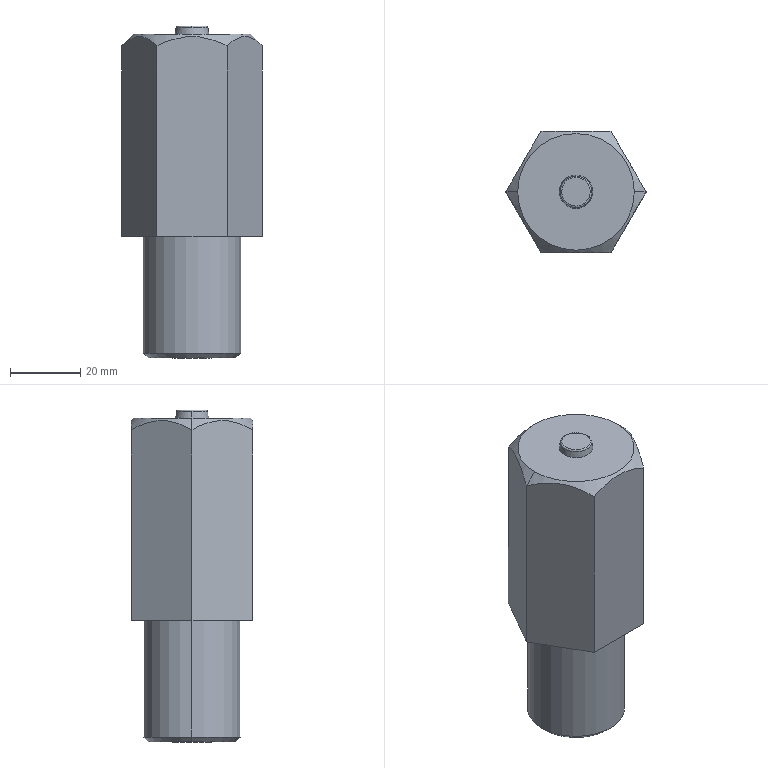Part | SolidWorks | features BaseBody 1 | 1 solid | 32 faces | box 39.97 x 34.615 x 94.615 mm | volume 79490 mm3 | plane 18 | cone 8 | cylinder 4 | spline 2 | commonest cylinder face diameters 11.347 x2 27.692 x2
STEP:
#1=CARTESIAN_POINT('',(-17.753,363.64,245.757));
#2=VERTEX_POINT('',#1);
#3=CARTESIAN_POINT('',(-13.229,359.115,245.757));
#4=VERTEX_POINT('',#3);
#5=CARTESIAN_POINT('',(-17.753,359.115,245.757));
#6=DIRECTION('',(0.,0.,-1.));
#7=DIRECTION('',(-1.,0.,0.));
#8=AXIS2_PLACEMENT_3D('',#5,#6,#7);
#9=CIRCLE('',#8,4.525);
#10=EDGE_CURVE('',#2,#4,#9,.T.);
#11=ORIENTED_EDGE('',*,*,#10,.F.);
#12=CARTESIAN_POINT('',(-17.753,363.183,246.154));
#13=VERTEX_POINT('',#12);
#14=CARTESIAN_POINT('',(-17.753,363.183,245.692));
#15=DIRECTION('',(1.,0.,0.));
#16=DIRECTION('',(0.,1.,0.));
#17=AXIS2_PLACEMENT_3D('',#14,#15,#16);
#18=CIRCLE('',#17,0.4615);
#19=EDGE_CURVE('',#2,#13,#18,.T.);
#20=ORIENTED_EDGE('',*,*,#19,.T.);
#21=CARTESIAN_POINT('',(-13.686,359.115,246.154));
#22=VERTEX_POINT('',#21);
#23=CARTESIAN_POINT('',(-17.753,363.183,246.154));
#24=CARTESIAN_POINT('',(-15.371,363.183,246.154));
#25=CARTESIAN_POINT('',(-13.686,361.498,246.154));
#26=CARTESIAN_POINT('',(-13.686,359.115,246.154));
#27=(BOUNDED_CURVE()B_SPLINE_CURVE(3,(#23,#24,#25,#26),.UNSPECIFIED.,.F.,.T.)B_SPLINE_CURVE_WITH_KNOTS((4,4),(0.,1.),.UNSPECIFIED.)CURVE()GEOMETRIC_REPRESENTATION_ITEM()RATIONAL_B_SPLINE_CURVE((1.,0.8047,0.8047,1.))REPRESENTATION_ITEM(''));
#28=EDGE_CURVE('',#13,#22,#27,.T.);
#29=ORIENTED_EDGE('',*,*,#28,.T.);
#30=CARTESIAN_POINT('',(-17.753,355.048,246.154));
#31=VERTEX_POINT('',#30);
#32=CARTESIAN_POINT('',(-13.686,359.115,246.154));
#33=CARTESIAN_POINT('',(-13.686,356.733,246.154));
#34=CARTESIAN_POINT('',(-15.371,355.048,246.154));
#35=CARTESIAN_POINT('',(-17.753,355.048,246.154));
#36=(BOUNDED_CURVE()B_SPLINE_CURVE(3,(#32,#33,#34,#35),.UNSPECIFIED.,.F.,.T.)B_SPLINE_CURVE_WITH_KNOTS((4,4),(0.,1.),.UNSPECIFIED.)CURVE()GEOMETRIC_REPRESENTATION_ITEM()RATIONAL_B_SPLINE_CURVE((1.,0.8047,0.8047,1.))REPRESENTATION_ITEM(''));
#37=EDGE_CURVE('',#22,#31,#36,.T.);
#38=ORIENTED_EDGE('',*,*,#37,.T.);
#39=CARTESIAN_POINT('',(-17.753,354.591,245.757));
#40=VERTEX_POINT('',#39);
#41=CARTESIAN_POINT('',(-17.753,355.048,245.692));
#42=DIRECTION('',(-1.,0.,0.));
#43=DIRECTION('',(0.,-1.,0.));
#44=AXIS2_PLACEMENT_3D('',#41,#42,#43);
#45=CIRCLE('',#44,0.4615);
#46=EDGE_CURVE('',#40,#31,#45,.T.);
#47=ORIENTED_EDGE('',*,*,#46,.F.);
#48=CARTESIAN_POINT('',(-17.753,359.115,245.757));
#49=DIRECTION('',(0.,0.,-1.));
#50=DIRECTION('',(-1.,0.,0.));
#51=AXIS2_PLACEMENT_3D('',#48,#49,#50);
#52=CIRCLE('',#51,4.525);
#53=EDGE_CURVE('',#4,#40,#52,.T.);
#54=ORIENTED_EDGE('',*,*,#53,.F.);
#55=EDGE_LOOP('',(#11,#20,#29,#38,#47,#54));
#56=FACE_OUTER_BOUND('',#55,.T.);
#57=CARTESIAN_POINT('',(-17.753,363.64,245.757));
#58=CARTESIAN_POINT('',(-8.704,363.64,245.757));
#59=CARTESIAN_POINT('',(-8.704,354.591,245.757));
#60=CARTESIAN_POINT('',(-17.753,354.591,245.757));
#61=CARTESIAN_POINT('',(-17.753,363.606,245.996));
#62=CARTESIAN_POINT('',(-8.771,363.606,245.996));
#63=CARTESIAN_POINT('',(-8.771,354.624,245.996));
#64=CARTESIAN_POINT('',(-17.753,354.624,245.996));
#65=CARTESIAN_POINT('',(-17.753,363.424,246.154));
#66=CARTESIAN_POINT('',(-9.136,363.424,246.154));
#67=CARTESIAN_POINT('',(-9.136,354.807,246.154));
#68=CARTESIAN_POINT('',(-17.753,354.807,246.154));
#69=CARTESIAN_POINT('',(-17.753,363.183,246.154));
#70=CARTESIAN_POINT('',(-9.618,363.183,246.154));
#71=CARTESIAN_POINT('',(-9.618,355.048,246.154));
#72=CARTESIAN_POINT('',(-17.753,355.048,246.154));
#73=(BOUNDED_SURFACE()B_SPLINE_SURFACE(3,3,((#57,#58,#59,#60),(#61,#62,#63,#64),(#65,#66,#67,#68),(#69,#70,#71,#72)),.UNSPECIFIED.,.F.,.F.,.T.)B_SPLINE_SURFACE_WITH_KNOTS((4,4),(4,4),(0.,1.),(0.,1.),.UNSPECIFIED.)GEOMETRIC_REPRESENTATION_ITEM()RATIONAL_B_SPLINE_SURFACE(((1.,0.3333,0.3333,1.),(0.8365,0.2788,0.2788,0.8365),(0.8365,0.2788,0.2788,0.8365),(1.,0.3333,0.3333,1.)))REPRESENTATION_ITEM('')SURFACE());
#74=ADVANCED_FACE('',(#56),#73,.T.);
#75=CARTESIAN_POINT('',(-3.907,359.115,152.954));
#76=VERTEX_POINT('',#75);
#77=CARTESIAN_POINT('',(-31.6,359.115,152.954));
#78=VERTEX_POINT('',#77);
#79=CARTESIAN_POINT('',(-17.753,359.115,152.954));
#80=DIRECTION('',(0.,0.,1.));
#81=DIRECTION('',(1.,0.,0.));
#82=AXIS2_PLACEMENT_3D('',#79,#80,#81);
#83=CIRCLE('',#82,13.846);
#84=EDGE_CURVE('',#76,#78,#83,.T.);
#85=ORIENTED_EDGE('',*,*,#84,.T.);
#86=CARTESIAN_POINT('',(-31.6,359.115,186.154));
#87=VERTEX_POINT('',#86);
#88=CARTESIAN_POINT('',(-31.6,359.115,151.538));
#89=DIRECTION('',(0.,0.,1.));
#90=VECTOR('',#89,1000.);
#91=LINE('',#88,#90);
#92=EDGE_CURVE('',#78,#87,#91,.T.);
#93=ORIENTED_EDGE('',*,*,#92,.T.);
#94=CARTESIAN_POINT('',(-3.907,359.115,186.154));
#95=VERTEX_POINT('',#94);
#96=CARTESIAN_POINT('',(-17.753,359.115,186.154));
#97=DIRECTION('',(0.,0.,-1.));
#98=DIRECTION('',(1.,0.,0.));
#99=AXIS2_PLACEMENT_3D('',#96,#97,#98);
#100=CIRCLE('',#99,13.846);
#101=EDGE_CURVE('',#87,#95,#100,.T.);
#102=ORIENTED_EDGE('',*,*,#101,.T.);
#103=CARTESIAN_POINT('',(-3.907,359.115,151.538));
#104=DIRECTION('',(0.,0.,1.));
#105=VECTOR('',#104,1000.);
#106=LINE('',#103,#105);
#107=EDGE_CURVE('',#76,#95,#106,.T.);
#108=ORIENTED_EDGE('',*,*,#107,.F.);
#109=EDGE_LOOP('',(#85,#93,#102,#108));
#110=FACE_OUTER_BOUND('',#109,.T.);
#111=CARTESIAN_POINT('',(-17.753,359.115,151.538));
#112=DIRECTION('',(0.,0.,1.));
#113=DIRECTION('',(1.,0.,0.));
#114=AXIS2_PLACEMENT_3D('',#111,#112,#113);
#115=CYLINDRICAL_SURFACE('',#114,13.846);
#116=ADVANCED_FACE('',(#110),#115,.T.);
#117=CARTESIAN_POINT('',(-5.323,359.115,151.538));
#118=VERTEX_POINT('',#117);
#119=CARTESIAN_POINT('',(-30.184,359.115,151.538));
#120=VERTEX_POINT('',#119);
#121=CARTESIAN_POINT('',(-17.753,359.115,151.538));
#122=DIRECTION('',(0.,0.,1.));
#123=DIRECTION('',(1.,0.,0.));
#124=AXIS2_PLACEMENT_3D('',#121,#122,#123);
#125=CIRCLE('',#124,12.43);
#126=EDGE_CURVE('',#118,#120,#125,.T.);
#127=ORIENTED_EDGE('',*,*,#126,.T.);
#128=CARTESIAN_POINT('',(-31.6,359.115,152.954));
#129=DIRECTION('',(-0.7071,0.,0.7071));
#130=VECTOR('',#129,1000.);
#131=LINE('',#128,#130);
#132=EDGE_CURVE('',#120,#78,#131,.T.);
#133=ORIENTED_EDGE('',*,*,#132,.T.);
#134=ORIENTED_EDGE('',*,*,#84,.F.);
#135=CARTESIAN_POINT('',(-3.907,359.115,152.954));
#136=DIRECTION('',(0.7071,0.,0.7071));
#137=VECTOR('',#136,1000.);
#138=LINE('',#135,#137);
#139=EDGE_CURVE('',#118,#76,#138,.T.);
#140=ORIENTED_EDGE('',*,*,#139,.F.);
#141=EDGE_LOOP('',(#127,#133,#134,#140));
#142=FACE_OUTER_BOUND('',#141,.T.);
#143=CARTESIAN_POINT('',(-17.753,359.115,152.954));
#144=DIRECTION('',(0.,0.,1.));
#145=DIRECTION('',(1.,0.,0.));
#146=AXIS2_PLACEMENT_3D('',#143,#144,#145);
#147=CONICAL_SURFACE('',#146,13.846,0.7854);
#148=ADVANCED_FACE('',(#142),#147,.T.);
#149=CARTESIAN_POINT('',(-34.369,359.115,243.846));
#150=VERTEX_POINT('',#149);
#151=CARTESIAN_POINT('',(-1.138,359.115,243.846));
#152=VERTEX_POINT('',#151);
#153=CARTESIAN_POINT('',(-17.753,359.115,243.846));
#154=DIRECTION('',(0.,0.,-1.));
#155=DIRECTION('',(-1.,0.,0.));
#156=AXIS2_PLACEMENT_3D('',#153,#154,#155);
#157=CIRCLE('',#156,16.615);
#158=EDGE_CURVE('',#150,#152,#157,.T.);
#159=ORIENTED_EDGE('',*,*,#158,.T.);
#160=CARTESIAN_POINT('',(2.232,359.115,240.476));
#161=VERTEX_POINT('',#160);
#162=CARTESIAN_POINT('',(2.252,359.115,240.456));
#163=DIRECTION('',(0.7071,0.,-0.7071));
#164=VECTOR('',#163,1000.);
#165=LINE('',#162,#164);
#166=EDGE_CURVE('',#152,#161,#165,.T.);
#167=ORIENTED_EDGE('',*,*,#166,.T.);
#168=CARTESIAN_POINT('',(-7.761,376.423,240.476));
#169=VERTEX_POINT('',#168);
#170=CARTESIAN_POINT('',(-7.761,376.423,240.476));
#171=CARTESIAN_POINT('',(-6.98,375.071,241.257));
#172=CARTESIAN_POINT('',(-6.182,373.688,241.921));
#173=CARTESIAN_POINT('',(-4.941,371.54,242.632));
#174=CARTESIAN_POINT('',(-4.521,370.811,242.821));
#175=CARTESIAN_POINT('',(-3.876,369.695,243.017));
#176=CARTESIAN_POINT('',(-3.659,369.319,243.067));
#177=CARTESIAN_POINT('',(-3.22,368.559,243.135));
#178=CARTESIAN_POINT('',(-3.001,368.179,243.153));
#179=CARTESIAN_POINT('',(-1.911,366.29,243.158));
#180=CARTESIAN_POINT('',(-1.053,364.805,242.893));
#181=CARTESIAN_POINT('',(0.6378,361.876,241.935));
#182=CARTESIAN_POINT('',(1.446,360.476,241.262));
#183=CARTESIAN_POINT('',(2.232,359.115,240.476));
#184=B_SPLINE_CURVE_WITH_KNOTS('',3,(#170,#171,#172,#173,#174,#175,#176,#177,#178,#179,#180,#181,#182,#183),.UNSPECIFIED.,.F.,.F.,(4,2,2,2,2,2,4),(0.,0.005161,0.007741,0.009032,0.01032,0.01548,0.02064),.UNSPECIFIED.);
#185=EDGE_CURVE('',#169,#161,#184,.T.);
#186=ORIENTED_EDGE('',*,*,#185,.F.);
#187=CARTESIAN_POINT('',(-27.746,376.423,240.476));
#188=VERTEX_POINT('',#187);
#189=CARTESIAN_POINT('',(-27.746,376.423,240.476));
#190=CARTESIAN_POINT('',(-26.185,376.423,241.257));
#191=CARTESIAN_POINT('',(-24.588,376.423,241.921));
#192=CARTESIAN_POINT('',(-22.107,376.423,242.632));
#193=CARTESIAN_POINT('',(-21.266,376.423,242.821));
#194=CARTESIAN_POINT('',(-19.977,376.423,243.017));
#195=CARTESIAN_POINT('',(-19.543,376.423,243.067));
#196=CARTESIAN_POINT('',(-18.665,376.423,243.135));
#197=CARTESIAN_POINT('',(-18.226,376.423,243.153));
#198=CARTESIAN_POINT('',(-16.046,376.423,243.158));
#199=CARTESIAN_POINT('',(-14.331,376.423,242.893));
#200=CARTESIAN_POINT('',(-10.949,376.423,241.935));
#201=CARTESIAN_POINT('',(-9.332,376.423,241.262));
#202=CARTESIAN_POINT('',(-7.761,376.423,240.476));
#203=B_SPLINE_CURVE_WITH_KNOTS('',3,(#189,#190,#191,#192,#193,#194,#195,#196,#197,#198,#199,#200,#201,#202),.UNSPECIFIED.,.F.,.F.,(4,2,2,2,2,2,4),(0.,0.005161,0.007741,0.009032,0.01032,0.01548,0.02064),.UNSPECIFIED.);
#204=EDGE_CURVE('',#188,#169,#203,.T.);
#205=ORIENTED_EDGE('',*,*,#204,.F.);
#206=CARTESIAN_POINT('',(-37.739,359.115,240.476));
#207=VERTEX_POINT('',#206);
#208=CARTESIAN_POINT('',(-37.739,359.115,240.476));
#209=CARTESIAN_POINT('',(-36.958,360.468,241.257));
#210=CARTESIAN_POINT('',(-36.16,361.851,241.921));
#211=CARTESIAN_POINT('',(-34.919,363.999,242.632));
#212=CARTESIAN_POINT('',(-34.499,364.728,242.821));
#213=CARTESIAN_POINT('',(-33.854,365.844,243.017));
#214=CARTESIAN_POINT('',(-33.637,366.219,243.067));
#215=CARTESIAN_POINT('',(-33.198,366.98,243.135));
#216=CARTESIAN_POINT('',(-32.979,367.36,243.153));
#217=CARTESIAN_POINT('',(-31.888,369.248,243.158));
#218=CARTESIAN_POINT('',(-31.031,370.733,242.893));
#219=CARTESIAN_POINT('',(-29.34,373.662,241.935));
#220=CARTESIAN_POINT('',(-28.531,375.063,241.262));
#221=CARTESIAN_POINT('',(-27.746,376.423,240.476));
#222=B_SPLINE_CURVE_WITH_KNOTS('',3,(#208,#209,#210,#211,#212,#213,#214,#215,#216,#217,#218,#219,#220,#221),.UNSPECIFIED.,.F.,.F.,(4,2,2,2,2,2,4),(0.,0.005161,0.007741,0.009032,0.01032,0.01548,0.02064),.UNSPECIFIED.);
#223=EDGE_CURVE('',#207,#188,#222,.T.);
#224=ORIENTED_EDGE('',*,*,#223,.F.);
#225=CARTESIAN_POINT('',(-37.759,359.115,240.456));
#226=DIRECTION('',(-0.7071,0.,-0.7071));
#227=VECTOR('',#226,1000.);
#228=LINE('',#225,#227);
#229=EDGE_CURVE('',#150,#207,#228,.T.);
#230=ORIENTED_EDGE('',*,*,#229,.F.);
#231=EDGE_LOOP('',(#159,#167,#186,#205,#224,#230));
#232=FACE_OUTER_BOUND('',#231,.T.);
#233=CARTESIAN_POINT('',(-17.753,359.115,240.456));
#234=DIRECTION('',(0.,0.,-1.));
#235=DIRECTION('',(-1.,0.,0.));
#236=AXIS2_PLACEMENT_3D('',#233,#234,#235);
#237=CONICAL_SURFACE('',#236,20.005,0.7854);
#238=ADVANCED_FACE('',(#232),#237,.T.);
#239=CARTESIAN_POINT('',(-12.08,359.115,151.538));
#240=VERTEX_POINT('',#239);
#241=CARTESIAN_POINT('',(-23.427,359.115,151.538));
#242=VERTEX_POINT('',#241);
#243=CARTESIAN_POINT('',(-17.753,359.115,151.538));
#244=DIRECTION('',(0.,0.,-1.));
#245=DIRECTION('',(1.,0.,0.));
#246=AXIS2_PLACEMENT_3D('',#243,#244,#245);
#247=CIRCLE('',#246,5.673);
#248=EDGE_CURVE('',#240,#242,#247,.T.);
#249=ORIENTED_EDGE('',*,*,#248,.T.);
#250=CARTESIAN_POINT('',(-23.427,359.115,160.935));
#251=VERTEX_POINT('',#250);
#252=CARTESIAN_POINT('',(-23.427,359.115,151.538));
#253=DIRECTION('',(0.,0.,1.));
#254=VECTOR('',#253,1000.);
#255=LINE('',#252,#254);
#256=EDGE_CURVE('',#242,#251,#255,.T.);
#257=ORIENTED_EDGE('',*,*,#256,.T.);
#258=CARTESIAN_POINT('',(-12.08,359.115,160.935));
#259=VERTEX_POINT('',#258);
#260=CARTESIAN_POINT('',(-17.753,359.115,160.935));
#261=DIRECTION('',(0.,0.,-1.));
#262=DIRECTION('',(1.,0.,0.));
#263=AXIS2_PLACEMENT_3D('',#260,#261,#262);
#264=CIRCLE('',#263,5.673);
#265=EDGE_CURVE('',#259,#251,#264,.T.);
#266=ORIENTED_EDGE('',*,*,#265,.F.);
#267=CARTESIAN_POINT('',(-12.08,359.115,151.538));
#268=DIRECTION('',(0.,0.,1.));
#269=VECTOR('',#268,1000.);
#270=LINE('',#267,#269);
#271=EDGE_CURVE('',#240,#259,#270,.T.);
#272=ORIENTED_EDGE('',*,*,#271,.F.);
#273=EDGE_LOOP('',(#249,#257,#266,#272));
#274=FACE_OUTER_BOUND('',#273,.T.);
#275=CARTESIAN_POINT('',(-17.753,359.115,151.538));
#276=DIRECTION('',(0.,0.,1.));
#277=DIRECTION('',(1.,0.,0.));
#278=AXIS2_PLACEMENT_3D('',#275,#276,#277);
#279=CYLINDRICAL_SURFACE('',#278,5.673);
#280=ADVANCED_FACE('',(#274),#279,.F.);
#281=CARTESIAN_POINT('',(-12.246,359.115,160.769));
#282=VERTEX_POINT('',#281);
#283=CARTESIAN_POINT('',(-23.261,359.115,160.769));
#284=VERTEX_POINT('',#283);
#285=CARTESIAN_POINT('',(-17.753,359.115,160.769));
#286=DIRECTION('',(0.,0.,1.));
#287=DIRECTION('',(1.,0.,0.));
#288=AXIS2_PLACEMENT_3D('',#285,#286,#287);
#289=CIRCLE('',#288,5.507);
#290=EDGE_CURVE('',#282,#284,#289,.T.);
#291=ORIENTED_EDGE('',*,*,#290,.T.);
#292=CARTESIAN_POINT('',(-23.427,359.115,160.935));
#293=DIRECTION('',(-0.7071,0.,0.7071));
#294=VECTOR('',#293,1000.);
#295=LINE('',#292,#294);
#296=EDGE_CURVE('',#284,#251,#295,.T.);
#297=ORIENTED_EDGE('',*,*,#296,.T.);
#298=CARTESIAN_POINT('',(-17.753,359.115,160.935));
#299=DIRECTION('',(0.,0.,-1.));
#300=DIRECTION('',(1.,0.,0.));
#301=AXIS2_PLACEMENT_3D('',#298,#299,#300);
#302=CIRCLE('',#301,5.673);
#303=EDGE_CURVE('',#251,#259,#302,.T.);
#304=ORIENTED_EDGE('',*,*,#303,.T.);
#305=CARTESIAN_POINT('',(-12.08,359.115,160.935));
#306=DIRECTION('',(0.7071,0.,0.7071));
#307=VECTOR('',#306,1000.);
#308=LINE('',#305,#307);
#309=EDGE_CURVE('',#282,#259,#308,.T.);
#310=ORIENTED_EDGE('',*,*,#309,.F.);
#311=EDGE_LOOP('',(#291,#297,#304,#310));
#312=FACE_OUTER_BOUND('',#311,.T.);
#313=CARTESIAN_POINT('',(-17.753,359.115,160.935));
#314=DIRECTION('',(0.,0.,1.));
#315=DIRECTION('',(1.,0.,0.));
#316=AXIS2_PLACEMENT_3D('',#313,#314,#315);
#317=CONICAL_SURFACE('',#316,5.673,0.7854);
#318=ADVANCED_FACE('',(#312),#317,.T.);
#319=CARTESIAN_POINT('',(-22.278,359.115,245.757));
#320=VERTEX_POINT('',#319);
#321=CARTESIAN_POINT('',(-17.753,359.115,245.757));
#322=DIRECTION('',(0.,0.,-1.));
#323=DIRECTION('',(-1.,0.,0.));
#324=AXIS2_PLACEMENT_3D('',#321,#322,#323);
#325=CIRCLE('',#324,4.525);
#326=EDGE_CURVE('',#320,#2,#325,.T.);
#327=ORIENTED_EDGE('',*,*,#326,.T.);
#328=ORIENTED_EDGE('',*,*,#10,.T.);
#329=CARTESIAN_POINT('',(-12.96,359.115,243.846));
#330=VERTEX_POINT('',#329);
#331=CARTESIAN_POINT('',(-12.96,359.115,243.846));
#332=DIRECTION('',(0.1392,0.,-0.9903));
#333=VECTOR('',#332,1000.);
#334=LINE('',#331,#333);
#335=EDGE_CURVE('',#4,#330,#334,.T.);
#336=ORIENTED_EDGE('',*,*,#335,.T.);
#337=CARTESIAN_POINT('',(-22.547,359.115,243.846));
#338=VERTEX_POINT('',#337);
#339=CARTESIAN_POINT('',(-17.753,359.115,243.846));
#340=DIRECTION('',(0.,0.,1.));
#341=DIRECTION('',(-1.,0.,0.));
#342=AXIS2_PLACEMENT_3D('',#339,#340,#341);
#343=CIRCLE('',#342,4.793);
#344=EDGE_CURVE('',#330,#338,#343,.T.);
#345=ORIENTED_EDGE('',*,*,#344,.T.);
#346=CARTESIAN_POINT('',(-22.547,359.115,243.846));
#347=DIRECTION('',(-0.1392,0.,-0.9903));
#348=VECTOR('',#347,1000.);
#349=LINE('',#346,#348);
#350=EDGE_CURVE('',#320,#338,#349,.T.);
#351=ORIENTED_EDGE('',*,*,#350,.F.);
#352=EDGE_LOOP('',(#327,#328,#336,#345,#351));
#353=FACE_OUTER_BOUND('',#352,.T.);
#354=CARTESIAN_POINT('',(-17.753,359.115,243.846));
#355=DIRECTION('',(0.,0.,-1.));
#356=DIRECTION('',(-1.,0.,0.));
#357=AXIS2_PLACEMENT_3D('',#354,#355,#356);
#358=CONICAL_SURFACE('',#357,4.793,0.1396);
#359=ADVANCED_FACE('',(#353),#358,.T.);
#360=ORIENTED_EDGE('',*,*,#92,.F.);
#361=CARTESIAN_POINT('',(-17.753,359.115,152.954));
#362=DIRECTION('',(0.,0.,1.));
#363=DIRECTION('',(1.,0.,0.));
#364=AXIS2_PLACEMENT_3D('',#361,#362,#363);
#365=CIRCLE('',#364,13.846);
#366=EDGE_CURVE('',#78,#76,#365,.T.);
#367=ORIENTED_EDGE('',*,*,#366,.T.);
#368=ORIENTED_EDGE('',*,*,#107,.T.);
#369=CARTESIAN_POINT('',(-17.753,359.115,186.154));
#370=DIRECTION('',(0.,0.,-1.));
#371=DIRECTION('',(1.,0.,0.));
#372=AXIS2_PLACEMENT_3D('',#369,#370,#371);
#373=CIRCLE('',#372,13.846);
#374=EDGE_CURVE('',#95,#87,#373,.T.);
#375=ORIENTED_EDGE('',*,*,#374,.T.);
#376=EDGE_LOOP('',(#360,#367,#368,#375));
#377=FACE_OUTER_BOUND('',#376,.T.);
#378=CARTESIAN_POINT('',(-17.753,359.115,151.538));
#379=DIRECTION('',(0.,0.,1.));
#380=DIRECTION('',(1.,0.,0.));
#381=AXIS2_PLACEMENT_3D('',#378,#379,#380);
#382=CYLINDRICAL_SURFACE('',#381,13.846);
#383=ADVANCED_FACE('',(#377),#382,.T.);
#384=ORIENTED_EDGE('',*,*,#374,.F.);
#385=ORIENTED_EDGE('',*,*,#101,.F.);
#386=EDGE_LOOP('',(#384,#385));
#387=FACE_BOUND('',#386,.T.);
#388=CARTESIAN_POINT('',(-7.761,376.423,186.154));
#389=VERTEX_POINT('',#388);
#390=CARTESIAN_POINT('',(-27.746,376.423,186.154));
#391=VERTEX_POINT('',#390);
#392=CARTESIAN_POINT('',(-17.753,376.423,186.154));
#393=DIRECTION('',(-1.,0.,0.));
#394=VECTOR('',#393,1000.);
#395=LINE('',#392,#394);
#396=EDGE_CURVE('',#389,#391,#395,.T.);
#397=ORIENTED_EDGE('',*,*,#396,.F.);
#398=CARTESIAN_POINT('',(2.232,359.115,186.154));
#399=VERTEX_POINT('',#398);
#400=CARTESIAN_POINT('',(2.232,359.115,186.154));
#401=DIRECTION('',(-0.5,0.866,0.));
#402=VECTOR('',#401,1000.);
#403=LINE('',#400,#402);
#404=EDGE_CURVE('',#399,#389,#403,.T.);
#405=ORIENTED_EDGE('',*,*,#404,.F.);
#406=CARTESIAN_POINT('',(-7.761,341.808,186.154));
#407=VERTEX_POINT('',#406);
#408=CARTESIAN_POINT('',(-7.761,341.808,186.154));
#409=DIRECTION('',(0.5,0.866,0.));
#410=VECTOR('',#409,1000.);
#411=LINE('',#408,#410);
#412=EDGE_CURVE('',#407,#399,#411,.T.);
#413=ORIENTED_EDGE('',*,*,#412,.F.);
#414=CARTESIAN_POINT('',(-27.746,341.808,186.154));
#415=VERTEX_POINT('',#414);
#416=CARTESIAN_POINT('',(-17.753,341.808,186.154));
#417=DIRECTION('',(1.,0.,0.));
#418=VECTOR('',#417,1000.);
#419=LINE('',#416,#418);
#420=EDGE_CURVE('',#415,#407,#419,.T.);
#421=ORIENTED_EDGE('',*,*,#420,.F.);
#422=CARTESIAN_POINT('',(-37.739,359.115,186.154));
#423=VERTEX_POINT('',#422);
#424=CARTESIAN_POINT('',(-37.739,359.115,186.154));
#425=DIRECTION('',(0.5,-0.866,0.));
#426=VECTOR('',#425,1000.);
#427=LINE('',#424,#426);
#428=EDGE_CURVE('',#423,#415,#427,.T.);
#429=ORIENTED_EDGE('',*,*,#428,.F.);
#430=CARTESIAN_POINT('',(-27.746,376.423,186.154));
#431=DIRECTION('',(-0.5,-0.866,0.));
#432=VECTOR('',#431,1000.);
#433=LINE('',#430,#432);
#434=EDGE_CURVE('',#391,#423,#433,.T.);
#435=ORIENTED_EDGE('',*,*,#434,.F.);
#436=EDGE_LOOP('',(#397,#405,#413,#421,#429,#435));
#437=FACE_OUTER_BOUND('',#436,.T.);
#438=CARTESIAN_POINT('',(-17.753,339.039,186.154));
#439=DIRECTION('',(0.,0.,1.));
#440=DIRECTION('',(1.,0.,0.));
#441=AXIS2_PLACEMENT_3D('',#438,#439,#440);
#442=PLANE('',#441);
#443=ADVANCED_FACE('',(#387,#437),#442,.F.);
#444=ORIENTED_EDGE('',*,*,#132,.F.);
#445=CARTESIAN_POINT('',(-17.753,359.115,151.538));
#446=DIRECTION('',(0.,0.,1.));
#447=DIRECTION('',(1.,0.,0.));
#448=AXIS2_PLACEMENT_3D('',#445,#446,#447);
#449=CIRCLE('',#448,12.43);
#450=EDGE_CURVE('',#120,#118,#449,.T.);
#451=ORIENTED_EDGE('',*,*,#450,.T.);
#452=ORIENTED_EDGE('',*,*,#139,.T.);
#453=ORIENTED_EDGE('',*,*,#366,.F.);
#454=EDGE_LOOP('',(#444,#451,#452,#453));
#455=FACE_OUTER_BOUND('',#454,.T.);
#456=CARTESIAN_POINT('',(-17.753,359.115,152.954));
#457=DIRECTION('',(0.,0.,1.));
#458=DIRECTION('',(1.,0.,0.));
#459=AXIS2_PLACEMENT_3D('',#456,#457,#458);
#460=CONICAL_SURFACE('',#459,13.846,0.7854);
#461=ADVANCED_FACE('',(#455),#460,.T.);
#462=CARTESIAN_POINT('',(-27.746,376.423,186.154));
#463=DIRECTION('',(0.,0.,-1.));
#464=VECTOR('',#463,1000.);
#465=LINE('',#462,#464);
#466=EDGE_CURVE('',#188,#391,#465,.T.);
#467=ORIENTED_EDGE('',*,*,#466,.T.);
#468=ORIENTED_EDGE('',*,*,#434,.T.);
#469=CARTESIAN_POINT('',(-37.739,359.115,186.154));
#470=DIRECTION('',(0.,0.,1.));
#471=VECTOR('',#470,1000.);
#472=LINE('',#469,#471);
#473=EDGE_CURVE('',#423,#207,#472,.T.);
#474=ORIENTED_EDGE('',*,*,#473,.T.);
#475=ORIENTED_EDGE('',*,*,#223,.T.);
#476=EDGE_LOOP('',(#467,#468,#474,#475));
#477=FACE_OUTER_BOUND('',#476,.T.);
#478=CARTESIAN_POINT('',(-27.746,376.423,186.154));
#479=DIRECTION('',(-0.866,0.5,0.));
#480=DIRECTION('',(-0.5,-0.866,0.));
#481=AXIS2_PLACEMENT_3D('',#478,#479,#480);
#482=PLANE('',#481);
#483=ADVANCED_FACE('',(#477),#482,.T.);
#484=CARTESIAN_POINT('',(-7.761,376.423,186.154));
#485=DIRECTION('',(0.,0.,-1.));
#486=VECTOR('',#485,1000.);
#487=LINE('',#484,#486);
#488=EDGE_CURVE('',#169,#389,#487,.T.);
#489=ORIENTED_EDGE('',*,*,#488,.T.);
#490=ORIENTED_EDGE('',*,*,#396,.T.);
#491=ORIENTED_EDGE('',*,*,#466,.F.);
#492=ORIENTED_EDGE('',*,*,#204,.T.);
#493=EDGE_LOOP('',(#489,#490,#491,#492));
#494=FACE_OUTER_BOUND('',#493,.T.);
#495=CARTESIAN_POINT('',(-7.761,376.423,186.154));
#496=DIRECTION('',(0.,1.,0.));
#497=DIRECTION('',(0.,0.,1.));
#498=AXIS2_PLACEMENT_3D('',#495,#496,#497);
#499=PLANE('',#498);
#500=ADVANCED_FACE('',(#494),#499,.T.);
#501=CARTESIAN_POINT('',(2.232,359.115,186.154));
#502=DIRECTION('',(0.,0.,-1.));
#503=VECTOR('',#502,1000.);
#504=LINE('',#501,#503);
#505=EDGE_CURVE('',#161,#399,#504,.T.);
#506=ORIENTED_EDGE('',*,*,#505,.T.);
#507=ORIENTED_EDGE('',*,*,#404,.T.);
#508=ORIENTED_EDGE('',*,*,#488,.F.);
#509=ORIENTED_EDGE('',*,*,#185,.T.);
#510=EDGE_LOOP('',(#506,#507,#508,#509));
#511=FACE_OUTER_BOUND('',#510,.T.);
#512=CARTESIAN_POINT('',(2.232,359.115,186.154));
#513=DIRECTION('',(0.866,0.5,0.));
#514=DIRECTION('',(-0.5,0.866,0.));
#515=AXIS2_PLACEMENT_3D('',#512,#513,#514);
#516=PLANE('',#515);
#517=ADVANCED_FACE('',(#511),#516,.T.);
#518=CARTESIAN_POINT('',(-7.761,341.808,240.476));
#519=VERTEX_POINT('',#518);
#520=CARTESIAN_POINT('',(-7.761,341.808,186.154));
#521=DIRECTION('',(0.,0.,-1.));
#522=VECTOR('',#521,1000.);
#523=LINE('',#520,#522);
#524=EDGE_CURVE('',#519,#407,#523,.T.);
#525=ORIENTED_EDGE('',*,*,#524,.T.);
#526=ORIENTED_EDGE('',*,*,#412,.T.);
#527=ORIENTED_EDGE('',*,*,#505,.F.);
#528=CARTESIAN_POINT('',(2.232,359.115,240.476));
#529=CARTESIAN_POINT('',(1.451,357.763,241.257));
#530=CARTESIAN_POINT('',(0.6526,356.38,241.921));
#531=CARTESIAN_POINT('',(-0.5878,354.232,242.632));
#532=CARTESIAN_POINT('',(-1.008,353.503,242.821));
#533=CARTESIAN_POINT('',(-1.653,352.387,243.017));
#534=CARTESIAN_POINT('',(-1.87,352.011,243.067));
#535=CARTESIAN_POINT('',(-2.309,351.251,243.135));
#536=CARTESIAN_POINT('',(-2.528,350.871,243.153));
#537=CARTESIAN_POINT('',(-3.619,348.983,243.158));
#538=CARTESIAN_POINT('',(-4.476,347.497,242.893));
#539=CARTESIAN_POINT('',(-6.167,344.569,241.935));
#540=CARTESIAN_POINT('',(-6.976,343.168,241.262));
#541=CARTESIAN_POINT('',(-7.761,341.808,240.476));
#542=B_SPLINE_CURVE_WITH_KNOTS('',3,(#528,#529,#530,#531,#532,#533,#534,#535,#536,#537,#538,#539,#540,#541),.UNSPECIFIED.,.F.,.F.,(4,2,2,2,2,2,4),(0.,0.005161,0.007741,0.009032,0.01032,0.01548,0.02064),.UNSPECIFIED.);
#543=EDGE_CURVE('',#161,#519,#542,.T.);
#544=ORIENTED_EDGE('',*,*,#543,.T.);
#545=EDGE_LOOP('',(#525,#526,#527,#544));
#546=FACE_OUTER_BOUND('',#545,.T.);
#547=CARTESIAN_POINT('',(-7.761,341.808,186.154));
#548=DIRECTION('',(0.866,-0.5,0.));
#549=DIRECTION('',(0.5,0.866,0.));
#550=AXIS2_PLACEMENT_3D('',#547,#548,#549);
#551=PLANE('',#550);
#552=ADVANCED_FACE('',(#546),#551,.T.);
#553=CARTESIAN_POINT('',(-27.746,341.808,240.476));
#554=VERTEX_POINT('',#553);
#555=CARTESIAN_POINT('',(-27.746,341.808,186.154));
#556=DIRECTION('',(0.,0.,-1.));
#557=VECTOR('',#556,1000.);
#558=LINE('',#555,#557);
#559=EDGE_CURVE('',#554,#415,#558,.T.);
#560=ORIENTED_EDGE('',*,*,#559,.T.);
#561=ORIENTED_EDGE('',*,*,#420,.T.);
#562=ORIENTED_EDGE('',*,*,#524,.F.);
#563=CARTESIAN_POINT('',(-7.761,341.808,240.476));
#564=CARTESIAN_POINT('',(-9.322,341.808,241.257));
#565=CARTESIAN_POINT('',(-10.919,341.808,241.921));
#566=CARTESIAN_POINT('',(-13.4,341.808,242.632));
#567=CARTESIAN_POINT('',(-14.241,341.808,242.821));
#568=CARTESIAN_POINT('',(-15.53,341.808,243.017));
#569=CARTESIAN_POINT('',(-15.964,341.808,243.067));
#570=CARTESIAN_POINT('',(-16.842,341.808,243.135));
#571=CARTESIAN_POINT('',(-17.281,341.808,243.153));
#572=CARTESIAN_POINT('',(-19.461,341.808,243.158));
#573=CARTESIAN_POINT('',(-21.176,341.808,242.893));
#574=CARTESIAN_POINT('',(-24.558,341.808,241.935));
#575=CARTESIAN_POINT('',(-26.175,341.808,241.262));
#576=CARTESIAN_POINT('',(-27.746,341.808,240.476));
#577=B_SPLINE_CURVE_WITH_KNOTS('',3,(#563,#564,#565,#566,#567,#568,#569,#570,#571,#572,#573,#574,#575,#576),.UNSPECIFIED.,.F.,.F.,(4,2,2,2,2,2,4),(0.,0.005161,0.007741,0.009032,0.01032,0.01548,0.02064),.UNSPECIFIED.);
#578=EDGE_CURVE('',#519,#554,#577,.T.);
#579=ORIENTED_EDGE('',*,*,#578,.T.);
#580=EDGE_LOOP('',(#560,#561,#562,#579));
#581=FACE_OUTER_BOUND('',#580,.T.);
#582=CARTESIAN_POINT('',(-27.746,341.808,186.154));
#583=DIRECTION('',(0.,-1.,0.));
#584=DIRECTION('',(0.,0.,-1.));
#585=AXIS2_PLACEMENT_3D('',#582,#583,#584);
#586=PLANE('',#585);
#587=ADVANCED_FACE('',(#581),#586,.T.);
#588=ORIENTED_EDGE('',*,*,#473,.F.);
#589=ORIENTED_EDGE('',*,*,#428,.T.);
#590=ORIENTED_EDGE('',*,*,#559,.F.);
#591=CARTESIAN_POINT('',(-27.746,341.808,240.476));
#592=CARTESIAN_POINT('',(-28.527,343.16,241.257));
#593=CARTESIAN_POINT('',(-29.325,344.543,241.921));
#594=CARTESIAN_POINT('',(-30.566,346.691,242.632));
#595=CARTESIAN_POINT('',(-30.986,347.42,242.821));
#596=CARTESIAN_POINT('',(-31.631,348.536,243.017));
#597=CARTESIAN_POINT('',(-31.848,348.912,243.067));
#598=CARTESIAN_POINT('',(-32.286,349.672,243.135));
#599=CARTESIAN_POINT('',(-32.506,350.052,243.153));
#600=CARTESIAN_POINT('',(-33.596,351.941,243.158));
#601=CARTESIAN_POINT('',(-34.454,353.426,242.893));
#602=CARTESIAN_POINT('',(-36.145,356.355,241.935));
#603=CARTESIAN_POINT('',(-36.953,357.755,241.262));
#604=CARTESIAN_POINT('',(-37.739,359.115,240.476));
#605=B_SPLINE_CURVE_WITH_KNOTS('',3,(#591,#592,#593,#594,#595,#596,#597,#598,#599,#600,#601,#602,#603,#604),.UNSPECIFIED.,.F.,.F.,(4,2,2,2,2,2,4),(0.,0.005161,0.007741,0.009032,0.01032,0.01548,0.02064),.UNSPECIFIED.);
#606=EDGE_CURVE('',#554,#207,#605,.T.);
#607=ORIENTED_EDGE('',*,*,#606,.T.);
#608=EDGE_LOOP('',(#588,#589,#590,#607));
#609=FACE_OUTER_BOUND('',#608,.T.);
#610=CARTESIAN_POINT('',(-37.739,359.115,186.154));
#611=DIRECTION('',(-0.866,-0.5,0.));
#612=DIRECTION('',(0.5,-0.866,0.));
#613=AXIS2_PLACEMENT_3D('',#610,#611,#612);
#614=PLANE('',#613);
#615=ADVANCED_FACE('',(#609),#614,.T.);
#616=ORIENTED_EDGE('',*,*,#248,.F.);
#617=CARTESIAN_POINT('',(-17.753,359.115,151.538));
#618=DIRECTION('',(0.,0.,-1.));
#619=DIRECTION('',(1.,0.,0.));
#620=AXIS2_PLACEMENT_3D('',#617,#618,#619);
#621=CIRCLE('',#620,5.673);
#622=EDGE_CURVE('',#242,#240,#621,.T.);
#623=ORIENTED_EDGE('',*,*,#622,.F.);
#624=EDGE_LOOP('',(#616,#623));
#625=FACE_BOUND('',#624,.T.);
#626=ORIENTED_EDGE('',*,*,#126,.F.);
#627=ORIENTED_EDGE('',*,*,#450,.F.);
#628=EDGE_LOOP('',(#626,#627));
#629=FACE_OUTER_BOUND('',#628,.T.);
#630=CARTESIAN_POINT('',(-17.753,346.685,151.538));
#631=DIRECTION('',(0.,0.,1.));
#632=DIRECTION('',(1.,0.,0.));
#633=AXIS2_PLACEMENT_3D('',#630,#631,#632);
#634=PLANE('',#633);
#635=ADVANCED_FACE('',(#625,#629),#634,.F.);
#636=ORIENTED_EDGE('',*,*,#166,.F.);
#637=CARTESIAN_POINT('',(-17.753,359.115,243.846));
#638=DIRECTION('',(0.,0.,-1.));
#639=DIRECTION('',(-1.,0.,0.));
#640=AXIS2_PLACEMENT_3D('',#637,#638,#639);
#641=CIRCLE('',#640,16.615);
#642=EDGE_CURVE('',#152,#150,#641,.T.);
#643=ORIENTED_EDGE('',*,*,#642,.T.);
#644=ORIENTED_EDGE('',*,*,#229,.T.);
#645=ORIENTED_EDGE('',*,*,#606,.F.);
#646=ORIENTED_EDGE('',*,*,#578,.F.);
#647=ORIENTED_EDGE('',*,*,#543,.F.);
#648=EDGE_LOOP('',(#636,#643,#644,#645,#646,#647));
#649=FACE_OUTER_BOUND('',#648,.T.);
#650=CARTESIAN_POINT('',(-17.753,359.115,240.456));
#651=DIRECTION('',(0.,0.,-1.));
#652=DIRECTION('',(-1.,0.,0.));
#653=AXIS2_PLACEMENT_3D('',#650,#651,#652);
#654=CONICAL_SURFACE('',#653,20.005,0.7854);
#655=ADVANCED_FACE('',(#649),#654,.T.);
#656=ORIENTED_EDGE('',*,*,#256,.F.);
#657=ORIENTED_EDGE('',*,*,#622,.T.);
#658=ORIENTED_EDGE('',*,*,#271,.T.);
#659=ORIENTED_EDGE('',*,*,#303,.F.);
#660=EDGE_LOOP('',(#656,#657,#658,#659));
#661=FACE_OUTER_BOUND('',#660,.T.);
#662=CARTESIAN_POINT('',(-17.753,359.115,151.538));
#663=DIRECTION('',(0.,0.,1.));
#664=DIRECTION('',(1.,0.,0.));
#665=AXIS2_PLACEMENT_3D('',#662,#663,#664);
#666=CYLINDRICAL_SURFACE('',#665,5.673);
#667=ADVANCED_FACE('',(#661),#666,.F.);
#668=CARTESIAN_POINT('',(-17.753,359.115,243.846));
#669=DIRECTION('',(0.,0.,1.));
#670=DIRECTION('',(-1.,0.,0.));
#671=AXIS2_PLACEMENT_3D('',#668,#669,#670);
#672=CIRCLE('',#671,4.793);
#673=EDGE_CURVE('',#338,#330,#672,.T.);
#674=ORIENTED_EDGE('',*,*,#673,.F.);
#675=ORIENTED_EDGE('',*,*,#344,.F.);
#676=EDGE_LOOP('',(#674,#675));
#677=FACE_BOUND('',#676,.T.);
#678=ORIENTED_EDGE('',*,*,#158,.F.);
#679=ORIENTED_EDGE('',*,*,#642,.F.);
#680=EDGE_LOOP('',(#678,#679));
#681=FACE_OUTER_BOUND('',#680,.T.);
#682=CARTESIAN_POINT('',(-17.753,359.115,243.846));
#683=DIRECTION('',(0.,0.,-1.));
#684=DIRECTION('',(-1.,0.,0.));
#685=AXIS2_PLACEMENT_3D('',#682,#683,#684);
#686=PLANE('',#685);
#687=ADVANCED_FACE('',(#677,#681),#686,.F.);
#688=ORIENTED_EDGE('',*,*,#296,.F.);
#689=CARTESIAN_POINT('',(-17.753,359.115,160.769));
#690=DIRECTION('',(0.,0.,1.));
#691=DIRECTION('',(1.,0.,0.));
#692=AXIS2_PLACEMENT_3D('',#689,#690,#691);
#693=CIRCLE('',#692,5.507);
#694=EDGE_CURVE('',#284,#282,#693,.T.);
#695=ORIENTED_EDGE('',*,*,#694,.T.);
#696=ORIENTED_EDGE('',*,*,#309,.T.);
#697=ORIENTED_EDGE('',*,*,#265,.T.);
#698=EDGE_LOOP('',(#688,#695,#696,#697));
#699=FACE_OUTER_BOUND('',#698,.T.);
#700=CARTESIAN_POINT('',(-17.753,359.115,160.935));
#701=DIRECTION('',(0.,0.,1.));
#702=DIRECTION('',(1.,0.,0.));
#703=AXIS2_PLACEMENT_3D('',#700,#701,#702);
#704=CONICAL_SURFACE('',#703,5.673,0.7854);
#705=ADVANCED_FACE('',(#699),#704,.T.);
#706=ORIENTED_EDGE('',*,*,#335,.F.);
#707=ORIENTED_EDGE('',*,*,#53,.T.);
#708=CARTESIAN_POINT('',(-17.753,359.115,245.757));
#709=DIRECTION('',(0.,0.,-1.));
#710=DIRECTION('',(-1.,0.,0.));
#711=AXIS2_PLACEMENT_3D('',#708,#709,#710);
#712=CIRCLE('',#711,4.525);
#713=EDGE_CURVE('',#40,#320,#712,.T.);
#714=ORIENTED_EDGE('',*,*,#713,.T.);
#715=ORIENTED_EDGE('',*,*,#350,.T.);
#716=ORIENTED_EDGE('',*,*,#673,.T.);
#717=EDGE_LOOP('',(#706,#707,#714,#715,#716));
#718=FACE_OUTER_BOUND('',#717,.T.);
#719=CARTESIAN_POINT('',(-17.753,359.115,243.846));
#720=DIRECTION('',(0.,0.,-1.));
#721=DIRECTION('',(-1.,0.,0.));
#722=AXIS2_PLACEMENT_3D('',#719,#720,#721);
#723=CONICAL_SURFACE('',#722,4.793,0.1396);
#724=ADVANCED_FACE('',(#718),#723,.T.);
#725=CARTESIAN_POINT('',(-17.753,363.112,160.769));
#726=VERTEX_POINT('',#725);
#727=CARTESIAN_POINT('',(-14.292,361.114,160.769));
#728=VERTEX_POINT('',#727);
#729=CARTESIAN_POINT('',(-17.753,363.112,160.769));
#730=DIRECTION('',(0.866,-0.5,0.));
#731=VECTOR('',#730,1000.);
#732=LINE('',#729,#731);
#733=EDGE_CURVE('',#726,#728,#732,.T.);
#734=ORIENTED_EDGE('',*,*,#733,.F.);
#735=CARTESIAN_POINT('',(-21.215,361.114,160.769));
#736=VERTEX_POINT('',#735);
#737=CARTESIAN_POINT('',(-21.215,361.114,160.769));
#738=DIRECTION('',(0.866,0.5,0.));
#739=VECTOR('',#738,1000.);
#740=LINE('',#737,#739);
#741=EDGE_CURVE('',#736,#726,#740,.T.);
#742=ORIENTED_EDGE('',*,*,#741,.F.);
#743=CARTESIAN_POINT('',(-21.215,357.117,160.769));
#744=VERTEX_POINT('',#743);
#745=CARTESIAN_POINT('',(-21.215,353.608,160.769));
#746=DIRECTION('',(0.,1.,0.));
#747=VECTOR('',#746,1000.);
#748=LINE('',#745,#747);
#749=EDGE_CURVE('',#744,#736,#748,.T.);
#750=ORIENTED_EDGE('',*,*,#749,.F.);
#751=CARTESIAN_POINT('',(-17.753,355.118,160.769));
#752=VERTEX_POINT('',#751);
#753=CARTESIAN_POINT('',(-17.753,355.118,160.769));
#754=DIRECTION('',(-0.866,0.5,0.));
#755=VECTOR('',#754,1000.);
#756=LINE('',#753,#755);
#757=EDGE_CURVE('',#752,#744,#756,.T.);
#758=ORIENTED_EDGE('',*,*,#757,.F.);
#759=CARTESIAN_POINT('',(-14.292,357.117,160.769));
#760=VERTEX_POINT('',#759);
#761=CARTESIAN_POINT('',(-14.292,357.117,160.769));
#762=DIRECTION('',(-0.866,-0.5,0.));
#763=VECTOR('',#762,1000.);
#764=LINE('',#761,#763);
#765=EDGE_CURVE('',#760,#752,#764,.T.);
#766=ORIENTED_EDGE('',*,*,#765,.F.);
#767=CARTESIAN_POINT('',(-14.292,353.608,160.769));
#768=DIRECTION('',(0.,-1.,0.));
#769=VECTOR('',#768,1000.);
#770=LINE('',#767,#769);
#771=EDGE_CURVE('',#728,#760,#770,.T.);
#772=ORIENTED_EDGE('',*,*,#771,.F.);
#773=EDGE_LOOP('',(#734,#742,#750,#758,#766,#772));
#774=FACE_BOUND('',#773,.T.);
#775=ORIENTED_EDGE('',*,*,#290,.F.);
#776=ORIENTED_EDGE('',*,*,#694,.F.);
#777=EDGE_LOOP('',(#775,#776));
#778=FACE_OUTER_BOUND('',#777,.T.);
#779=CARTESIAN_POINT('',(-17.753,353.608,160.769));
#780=DIRECTION('',(0.,0.,1.));
#781=DIRECTION('',(1.,0.,0.));
#782=AXIS2_PLACEMENT_3D('',#779,#780,#781);
#783=PLANE('',#782);
#784=ADVANCED_FACE('',(#774,#778),#783,.F.);
#785=ORIENTED_EDGE('',*,*,#19,.F.);
#786=ORIENTED_EDGE('',*,*,#326,.F.);
#787=ORIENTED_EDGE('',*,*,#713,.F.);
#788=ORIENTED_EDGE('',*,*,#46,.T.);
#789=CARTESIAN_POINT('',(-17.753,355.048,246.154));
#790=CARTESIAN_POINT('',(-25.889,355.048,246.154));
#791=CARTESIAN_POINT('',(-25.889,363.183,246.154));
#792=CARTESIAN_POINT('',(-17.753,363.183,246.154));
#793=(BOUNDED_CURVE()B_SPLINE_CURVE(3,(#789,#790,#791,#792),.UNSPECIFIED.,.F.,.F.)B_SPLINE_CURVE_WITH_KNOTS((4,4),(0.,1.),.UNSPECIFIED.)CURVE()GEOMETRIC_REPRESENTATION_ITEM()RATIONAL_B_SPLINE_CURVE((1.,0.3333,0.3333,1.))REPRESENTATION_ITEM(''));
#794=EDGE_CURVE('',#31,#13,#793,.T.);
#795=ORIENTED_EDGE('',*,*,#794,.T.);
#796=EDGE_LOOP('',(#785,#786,#787,#788,#795));
#797=FACE_OUTER_BOUND('',#796,.T.);
#798=CARTESIAN_POINT('',(-17.753,354.591,245.757));
#799=CARTESIAN_POINT('',(-26.803,354.591,245.757));
#800=CARTESIAN_POINT('',(-26.803,363.64,245.757));
#801=CARTESIAN_POINT('',(-17.753,363.64,245.757));
#802=CARTESIAN_POINT('',(-17.753,354.624,245.996));
#803=CARTESIAN_POINT('',(-26.736,354.624,245.996));
#804=CARTESIAN_POINT('',(-26.736,363.606,245.996));
#805=CARTESIAN_POINT('',(-17.753,363.606,245.996));
#806=CARTESIAN_POINT('',(-17.753,354.807,246.154));
#807=CARTESIAN_POINT('',(-26.371,354.807,246.154));
#808=CARTESIAN_POINT('',(-26.371,363.424,246.154));
#809=CARTESIAN_POINT('',(-17.753,363.424,246.154));
#810=CARTESIAN_POINT('',(-17.753,355.048,246.154));
#811=CARTESIAN_POINT('',(-25.889,355.048,246.154));
#812=CARTESIAN_POINT('',(-25.889,363.183,246.154));
#813=CARTESIAN_POINT('',(-17.753,363.183,246.154));
#814=(BOUNDED_SURFACE()B_SPLINE_SURFACE(3,3,((#798,#799,#800,#801),(#802,#803,#804,#805),(#806,#807,#808,#809),(#810,#811,#812,#813)),.UNSPECIFIED.,.F.,.F.,.T.)B_SPLINE_SURFACE_WITH_KNOTS((4,4),(4,4),(0.,1.),(0.,1.),.UNSPECIFIED.)GEOMETRIC_REPRESENTATION_ITEM()RATIONAL_B_SPLINE_SURFACE(((1.,0.3333,0.3333,1.),(0.8365,0.2788,0.2788,0.8365),(0.8365,0.2788,0.2788,0.8365),(1.,0.3333,0.3333,1.)))REPRESENTATION_ITEM('')SURFACE());
#815=ADVANCED_FACE('',(#797),#814,.T.);
#816=CARTESIAN_POINT('',(-14.292,357.117,165.385));
#817=VERTEX_POINT('',#816);
#818=CARTESIAN_POINT('',(-14.292,357.117,165.385));
#819=DIRECTION('',(0.,0.,1.));
#820=VECTOR('',#819,1000.);
#821=LINE('',#818,#820);
#822=EDGE_CURVE('',#760,#817,#821,.T.);
#823=ORIENTED_EDGE('',*,*,#822,.T.);
#824=CARTESIAN_POINT('',(-14.292,361.114,165.385));
#825=VERTEX_POINT('',#824);
#826=CARTESIAN_POINT('',(-14.292,357.117,165.385));
#827=DIRECTION('',(0.,1.,0.));
#828=VECTOR('',#827,1000.);
#829=LINE('',#826,#828);
#830=EDGE_CURVE('',#817,#825,#829,.T.);
#831=ORIENTED_EDGE('',*,*,#830,.T.);
#832=CARTESIAN_POINT('',(-14.292,361.114,165.385));
#833=DIRECTION('',(0.,0.,-1.));
#834=VECTOR('',#833,1000.);
#835=LINE('',#832,#834);
#836=EDGE_CURVE('',#825,#728,#835,.T.);
#837=ORIENTED_EDGE('',*,*,#836,.T.);
#838=ORIENTED_EDGE('',*,*,#771,.T.);
#839=EDGE_LOOP('',(#823,#831,#837,#838));
#840=FACE_OUTER_BOUND('',#839,.T.);
#841=CARTESIAN_POINT('',(-14.292,357.117,165.385));
#842=DIRECTION('',(-1.,0.,0.));
#843=DIRECTION('',(0.,0.,1.));
#844=AXIS2_PLACEMENT_3D('',#841,#842,#843);
#845=PLANE('',#844);
#846=ADVANCED_FACE('',(#840),#845,.T.);
#847=ORIENTED_EDGE('',*,*,#836,.F.);
#848=CARTESIAN_POINT('',(-17.753,363.112,165.385));
#849=VERTEX_POINT('',#848);
#850=CARTESIAN_POINT('',(-14.292,361.114,165.385));
#851=DIRECTION('',(-0.866,0.5,0.));
#852=VECTOR('',#851,1000.);
#853=LINE('',#850,#852);
#854=EDGE_CURVE('',#825,#849,#853,.T.);
#855=ORIENTED_EDGE('',*,*,#854,.T.);
#856=CARTESIAN_POINT('',(-17.753,363.112,165.385));
#857=DIRECTION('',(0.,0.,-1.));
#858=VECTOR('',#857,1000.);
#859=LINE('',#856,#858);
#860=EDGE_CURVE('',#849,#726,#859,.T.);
#861=ORIENTED_EDGE('',*,*,#860,.T.);
#862=ORIENTED_EDGE('',*,*,#733,.T.);
#863=EDGE_LOOP('',(#847,#855,#861,#862));
#864=FACE_OUTER_BOUND('',#863,.T.);
#865=CARTESIAN_POINT('',(-14.292,361.114,165.385));
#866=DIRECTION('',(-0.5,-0.866,0.));
#867=DIRECTION('',(0.866,-0.5,0.));
#868=AXIS2_PLACEMENT_3D('',#865,#866,#867);
#869=PLANE('',#868);
#870=ADVANCED_FACE('',(#864),#869,.T.);
#871=ORIENTED_EDGE('',*,*,#860,.F.);
#872=CARTESIAN_POINT('',(-21.215,361.114,165.385));
#873=VERTEX_POINT('',#872);
#874=CARTESIAN_POINT('',(-17.753,363.112,165.385));
#875=DIRECTION('',(-0.866,-0.5,0.));
#876=VECTOR('',#875,1000.);
#877=LINE('',#874,#876);
#878=EDGE_CURVE('',#849,#873,#877,.T.);
#879=ORIENTED_EDGE('',*,*,#878,.T.);
#880=CARTESIAN_POINT('',(-21.215,361.114,165.385));
#881=DIRECTION('',(0.,0.,-1.));
#882=VECTOR('',#881,1000.);
#883=LINE('',#880,#882);
#884=EDGE_CURVE('',#873,#736,#883,.T.);
#885=ORIENTED_EDGE('',*,*,#884,.T.);
#886=ORIENTED_EDGE('',*,*,#741,.T.);
#887=EDGE_LOOP('',(#871,#879,#885,#886));
#888=FACE_OUTER_BOUND('',#887,.T.);
#889=CARTESIAN_POINT('',(-17.753,363.112,165.385));
#890=DIRECTION('',(0.5,-0.866,0.));
#891=DIRECTION('',(0.866,0.5,0.));
#892=AXIS2_PLACEMENT_3D('',#889,#890,#891);
#893=PLANE('',#892);
#894=ADVANCED_FACE('',(#888),#893,.T.);
#895=ORIENTED_EDGE('',*,*,#884,.F.);
#896=CARTESIAN_POINT('',(-21.215,357.117,165.385));
#897=VERTEX_POINT('',#896);
#898=CARTESIAN_POINT('',(-21.215,361.114,165.385));
#899=DIRECTION('',(0.,-1.,0.));
#900=VECTOR('',#899,1000.);
#901=LINE('',#898,#900);
#902=EDGE_CURVE('',#873,#897,#901,.T.);
#903=ORIENTED_EDGE('',*,*,#902,.T.);
#904=CARTESIAN_POINT('',(-21.215,357.117,165.385));
#905=DIRECTION('',(0.,0.,-1.));
#906=VECTOR('',#905,1000.);
#907=LINE('',#904,#906);
#908=EDGE_CURVE('',#897,#744,#907,.T.);
#909=ORIENTED_EDGE('',*,*,#908,.T.);
#910=ORIENTED_EDGE('',*,*,#749,.T.);
#911=EDGE_LOOP('',(#895,#903,#909,#910));
#912=FACE_OUTER_BOUND('',#911,.T.);
#913=CARTESIAN_POINT('',(-21.215,361.114,165.385));
#914=DIRECTION('',(1.,0.,0.));
#915=DIRECTION('',(0.,0.,-1.));
#916=AXIS2_PLACEMENT_3D('',#913,#914,#915);
#917=PLANE('',#916);
#918=ADVANCED_FACE('',(#912),#917,.T.);
#919=ORIENTED_EDGE('',*,*,#908,.F.);
#920=CARTESIAN_POINT('',(-17.753,355.118,165.385));
#921=VERTEX_POINT('',#920);
#922=CARTESIAN_POINT('',(-21.215,357.117,165.385));
#923=DIRECTION('',(0.866,-0.5,0.));
#924=VECTOR('',#923,1000.);
#925=LINE('',#922,#924);
#926=EDGE_CURVE('',#897,#921,#925,.T.);
#927=ORIENTED_EDGE('',*,*,#926,.T.);
#928=CARTESIAN_POINT('',(-17.753,355.118,165.385));
#929=DIRECTION('',(0.,0.,-1.));
#930=VECTOR('',#929,1000.);
#931=LINE('',#928,#930);
#932=EDGE_CURVE('',#921,#752,#931,.T.);
#933=ORIENTED_EDGE('',*,*,#932,.T.);
#934=ORIENTED_EDGE('',*,*,#757,.T.);
#935=EDGE_LOOP('',(#919,#927,#933,#934));
#936=FACE_OUTER_BOUND('',#935,.T.);
#937=CARTESIAN_POINT('',(-21.215,357.117,165.385));
#938=DIRECTION('',(0.5,0.866,0.));
#939=DIRECTION('',(-0.866,0.5,0.));
#940=AXIS2_PLACEMENT_3D('',#937,#938,#939);
#941=PLANE('',#940);
#942=ADVANCED_FACE('',(#936),#941,.T.);
#943=ORIENTED_EDGE('',*,*,#932,.F.);
#944=CARTESIAN_POINT('',(-17.753,355.118,165.385));
#945=DIRECTION('',(0.866,0.5,0.));
#946=VECTOR('',#945,1000.);
#947=LINE('',#944,#946);
#948=EDGE_CURVE('',#921,#817,#947,.T.);
#949=ORIENTED_EDGE('',*,*,#948,.T.);
#950=ORIENTED_EDGE('',*,*,#822,.F.);
#951=ORIENTED_EDGE('',*,*,#765,.T.);
#952=EDGE_LOOP('',(#943,#949,#950,#951));
#953=FACE_OUTER_BOUND('',#952,.T.);
#954=CARTESIAN_POINT('',(-17.753,355.118,165.385));
#955=DIRECTION('',(-0.5,0.866,0.));
#956=DIRECTION('',(-0.866,-0.5,0.));
#957=AXIS2_PLACEMENT_3D('',#954,#955,#956);
#958=PLANE('',#957);
#959=ADVANCED_FACE('',(#953),#958,.T.);
#960=ORIENTED_EDGE('',*,*,#878,.F.);
#961=ORIENTED_EDGE('',*,*,#854,.F.);
#962=ORIENTED_EDGE('',*,*,#830,.F.);
#963=ORIENTED_EDGE('',*,*,#948,.F.);
#964=ORIENTED_EDGE('',*,*,#926,.F.);
#965=ORIENTED_EDGE('',*,*,#902,.F.);
#966=EDGE_LOOP('',(#960,#961,#962,#963,#964,#965));
#967=FACE_OUTER_BOUND('',#966,.T.);
#968=CARTESIAN_POINT('',(-17.753,359.115,165.385));
#969=DIRECTION('',(0.,0.,1.));
#970=DIRECTION('',(1.,0.,0.));
#971=AXIS2_PLACEMENT_3D('',#968,#969,#970);
#972=PLANE('',#971);
#973=ADVANCED_FACE('',(#967),#972,.F.);
#974=ORIENTED_EDGE('',*,*,#37,.F.);
#975=ORIENTED_EDGE('',*,*,#28,.F.);
#976=ORIENTED_EDGE('',*,*,#794,.F.);
#977=EDGE_LOOP('',(#974,#975,#976));
#978=FACE_OUTER_BOUND('',#977,.T.);
#979=CARTESIAN_POINT('',(-17.753,359.115,246.154));
#980=DIRECTION('',(0.,0.,-1.));
#981=DIRECTION('',(-1.,0.,0.));
#982=AXIS2_PLACEMENT_3D('',#979,#980,#981);
#983=PLANE('',#982);
#984=ADVANCED_FACE('',(#978),#983,.F.);
#985=CLOSED_SHELL('',(#74,#116,#148,#238,#280,#318,#359,#383,#443,#461,#483,#500,#517,#552,#587,#615,#635,#655,#667,#687,#705,#724,#784,#815,#846,#870,#894,#918,#942,#959,#973,#984));
#986=MANIFOLD_SOLID_BREP('',#985);
#987=CARTESIAN_POINT('',(0.,0.,0.));
#988=DIRECTION('',(0.,0.,1.));
#989=DIRECTION('',(1.,0.,0.));
#990=AXIS2_PLACEMENT_3D('',#987,#988,#989);
#991=(LENGTH_UNIT()NAMED_UNIT(*)SI_UNIT(.MILLI.,.METRE.));
#992=UNCERTAINTY_MEASURE_WITH_UNIT(LENGTH_MEASURE(0.00001),#991,'','');
#993=(NAMED_UNIT(*)PLANE_ANGLE_UNIT()SI_UNIT($,.RADIAN.));
#994=(NAMED_UNIT(*)SI_UNIT($,.STERADIAN.)SOLID_ANGLE_UNIT());
#995=(GEOMETRIC_REPRESENTATION_CONTEXT(3)GLOBAL_UNCERTAINTY_ASSIGNED_CONTEXT((#992))GLOBAL_UNIT_ASSIGNED_CONTEXT((#991,#993,#994))REPRESENTATION_CONTEXT('',''));
#996=ADVANCED_BREP_SHAPE_REPRESENTATION('',(#986,#990),#995);